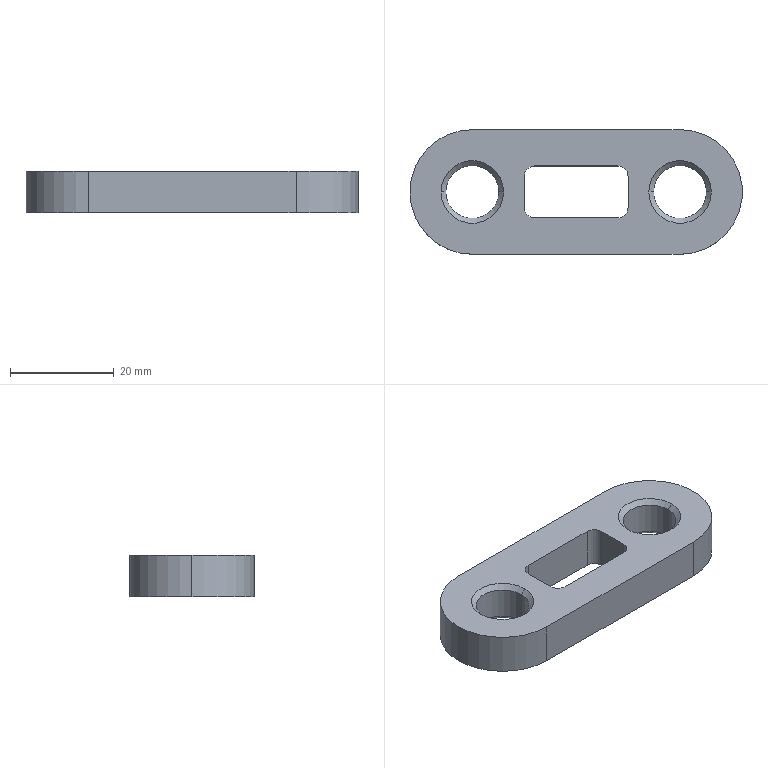Part | SolidWorks | features MirrorPattern 2, 3DProfileFeature 1, Extrusion 1, HoleWzd 1 | 1 solid | 27 faces | box 64 x 24 x 8 mm | volume 8361 mm3 | cylinder 11 | cone 8 | plane 8 | commonest cylinder face diameters 4 x4 10.2 x4 24 x3
STEP:
#1=CARTESIAN_POINT('',(45.1,0.,-3.075));
#2=VERTEX_POINT('',#1);
#3=CARTESIAN_POINT('',(34.9,0.,-3.075));
#4=VERTEX_POINT('',#3);
#5=CARTESIAN_POINT('',(40.,0.,-3.075));
#6=DIRECTION('',(0.,0.,-1.));
#7=DIRECTION('',(-1.,0.,0.));
#8=AXIS2_PLACEMENT_3D('',#5,#6,#7);
#9=CIRCLE('',#8,5.1);
#10=EDGE_CURVE('',#2,#4,#9,.T.);
#11=ORIENTED_EDGE('',*,*,#10,.F.);
#12=CARTESIAN_POINT('',(46.025,0.,-4.));
#13=VERTEX_POINT('',#12);
#14=CARTESIAN_POINT('',(46.025,0.,-4.));
#15=DIRECTION('',(0.7071,0.,-0.7071));
#16=VECTOR('',#15,1000.);
#17=LINE('',#14,#16);
#18=EDGE_CURVE('',#2,#13,#17,.T.);
#19=ORIENTED_EDGE('',*,*,#18,.T.);
#20=CARTESIAN_POINT('',(33.975,0.,-4.));
#21=VERTEX_POINT('',#20);
#22=CARTESIAN_POINT('',(40.,0.,-4.));
#23=DIRECTION('',(0.,0.,-1.));
#24=DIRECTION('',(-1.,0.,0.));
#25=AXIS2_PLACEMENT_3D('',#22,#23,#24);
#26=CIRCLE('',#25,6.025);
#27=EDGE_CURVE('',#13,#21,#26,.T.);
#28=ORIENTED_EDGE('',*,*,#27,.T.);
#29=CARTESIAN_POINT('',(33.975,0.,-4.));
#30=DIRECTION('',(-0.7071,0.,-0.7071));
#31=VECTOR('',#30,1000.);
#32=LINE('',#29,#31);
#33=EDGE_CURVE('',#4,#21,#32,.T.);
#34=ORIENTED_EDGE('',*,*,#33,.F.);
#35=EDGE_LOOP('',(#11,#19,#28,#34));
#36=FACE_OUTER_BOUND('',#35,.T.);
#37=CARTESIAN_POINT('',(40.,0.,-4.));
#38=DIRECTION('',(0.,0.,-1.));
#39=DIRECTION('',(-1.,0.,0.));
#40=AXIS2_PLACEMENT_3D('',#37,#38,#39);
#41=CONICAL_SURFACE('',#40,6.025,0.7854);
#42=ADVANCED_FACE('',(#36),#41,.F.);
#43=CARTESIAN_POINT('',(34.9,0.,3.075));
#44=VERTEX_POINT('',#43);
#45=CARTESIAN_POINT('',(45.1,0.,3.075));
#46=VERTEX_POINT('',#45);
#47=CARTESIAN_POINT('',(40.,0.,3.075));
#48=DIRECTION('',(0.,0.,1.));
#49=DIRECTION('',(1.,0.,0.));
#50=AXIS2_PLACEMENT_3D('',#47,#48,#49);
#51=CIRCLE('',#50,5.1);
#52=EDGE_CURVE('',#44,#46,#51,.T.);
#53=ORIENTED_EDGE('',*,*,#52,.F.);
#54=CARTESIAN_POINT('',(33.975,0.,4.));
#55=VERTEX_POINT('',#54);
#56=CARTESIAN_POINT('',(33.975,0.,4.));
#57=DIRECTION('',(-0.7071,0.,0.7071));
#58=VECTOR('',#57,1000.);
#59=LINE('',#56,#58);
#60=EDGE_CURVE('',#44,#55,#59,.T.);
#61=ORIENTED_EDGE('',*,*,#60,.T.);
#62=CARTESIAN_POINT('',(46.025,0.,4.));
#63=VERTEX_POINT('',#62);
#64=CARTESIAN_POINT('',(40.,0.,4.));
#65=DIRECTION('',(0.,0.,1.));
#66=DIRECTION('',(1.,0.,0.));
#67=AXIS2_PLACEMENT_3D('',#64,#65,#66);
#68=CIRCLE('',#67,6.025);
#69=EDGE_CURVE('',#55,#63,#68,.T.);
#70=ORIENTED_EDGE('',*,*,#69,.T.);
#71=CARTESIAN_POINT('',(46.025,0.,4.));
#72=DIRECTION('',(0.7071,0.,0.7071));
#73=VECTOR('',#72,1000.);
#74=LINE('',#71,#73);
#75=EDGE_CURVE('',#46,#63,#74,.T.);
#76=ORIENTED_EDGE('',*,*,#75,.F.);
#77=EDGE_LOOP('',(#53,#61,#70,#76));
#78=FACE_OUTER_BOUND('',#77,.T.);
#79=CARTESIAN_POINT('',(40.,0.,4.));
#80=DIRECTION('',(0.,0.,1.));
#81=DIRECTION('',(1.,0.,0.));
#82=AXIS2_PLACEMENT_3D('',#79,#80,#81);
#83=CONICAL_SURFACE('',#82,6.025,0.7854);
#84=ADVANCED_FACE('',(#78),#83,.F.);
#85=ORIENTED_EDGE('',*,*,#10,.T.);
#86=CARTESIAN_POINT('',(34.9,0.,4.));
#87=DIRECTION('',(0.,0.,1.));
#88=VECTOR('',#87,1000.);
#89=LINE('',#86,#88);
#90=EDGE_CURVE('',#4,#44,#89,.T.);
#91=ORIENTED_EDGE('',*,*,#90,.T.);
#92=ORIENTED_EDGE('',*,*,#52,.T.);
#93=CARTESIAN_POINT('',(45.1,0.,4.));
#94=DIRECTION('',(0.,0.,1.));
#95=VECTOR('',#94,1000.);
#96=LINE('',#93,#95);
#97=EDGE_CURVE('',#2,#46,#96,.T.);
#98=ORIENTED_EDGE('',*,*,#97,.F.);
#99=EDGE_LOOP('',(#85,#91,#92,#98));
#100=FACE_OUTER_BOUND('',#99,.T.);
#101=CARTESIAN_POINT('',(40.,0.,4.));
#102=DIRECTION('',(0.,0.,1.));
#103=DIRECTION('',(1.,0.,0.));
#104=AXIS2_PLACEMENT_3D('',#101,#102,#103);
#105=CYLINDRICAL_SURFACE('',#104,5.1);
#106=ADVANCED_FACE('',(#100),#105,.F.);
#107=CARTESIAN_POINT('',(5.1,0.,-3.075));
#108=VERTEX_POINT('',#107);
#109=CARTESIAN_POINT('',(-5.1,0.,-3.075));
#110=VERTEX_POINT('',#109);
#111=CARTESIAN_POINT('',(0.,0.,-3.075));
#112=DIRECTION('',(0.,0.,-1.));
#113=DIRECTION('',(-1.,0.,0.));
#114=AXIS2_PLACEMENT_3D('',#111,#112,#113);
#115=CIRCLE('',#114,5.1);
#116=EDGE_CURVE('',#108,#110,#115,.T.);
#117=ORIENTED_EDGE('',*,*,#116,.F.);
#118=CARTESIAN_POINT('',(6.025,0.,-4.));
#119=VERTEX_POINT('',#118);
#120=CARTESIAN_POINT('',(6.025,0.,-4.));
#121=DIRECTION('',(0.7071,0.,-0.7071));
#122=VECTOR('',#121,1000.);
#123=LINE('',#120,#122);
#124=EDGE_CURVE('',#108,#119,#123,.T.);
#125=ORIENTED_EDGE('',*,*,#124,.T.);
#126=CARTESIAN_POINT('',(-6.025,0.,-4.));
#127=VERTEX_POINT('',#126);
#128=CARTESIAN_POINT('',(0.,0.,-4.));
#129=DIRECTION('',(0.,0.,-1.));
#130=DIRECTION('',(-1.,0.,0.));
#131=AXIS2_PLACEMENT_3D('',#128,#129,#130);
#132=CIRCLE('',#131,6.025);
#133=EDGE_CURVE('',#119,#127,#132,.T.);
#134=ORIENTED_EDGE('',*,*,#133,.T.);
#135=CARTESIAN_POINT('',(-6.025,0.,-4.));
#136=DIRECTION('',(-0.7071,0.,-0.7071));
#137=VECTOR('',#136,1000.);
#138=LINE('',#135,#137);
#139=EDGE_CURVE('',#110,#127,#138,.T.);
#140=ORIENTED_EDGE('',*,*,#139,.F.);
#141=EDGE_LOOP('',(#117,#125,#134,#140));
#142=FACE_OUTER_BOUND('',#141,.T.);
#143=CARTESIAN_POINT('',(0.,0.,-4.));
#144=DIRECTION('',(0.,0.,-1.));
#145=DIRECTION('',(-1.,0.,0.));
#146=AXIS2_PLACEMENT_3D('',#143,#144,#145);
#147=CONICAL_SURFACE('',#146,6.025,0.7854);
#148=ADVANCED_FACE('',(#142),#147,.F.);
#149=CARTESIAN_POINT('',(-5.1,0.,3.075));
#150=VERTEX_POINT('',#149);
#151=CARTESIAN_POINT('',(5.1,0.,3.075));
#152=VERTEX_POINT('',#151);
#153=CARTESIAN_POINT('',(0.,0.,3.075));
#154=DIRECTION('',(0.,0.,1.));
#155=DIRECTION('',(1.,0.,0.));
#156=AXIS2_PLACEMENT_3D('',#153,#154,#155);
#157=CIRCLE('',#156,5.1);
#158=EDGE_CURVE('',#150,#152,#157,.T.);
#159=ORIENTED_EDGE('',*,*,#158,.F.);
#160=CARTESIAN_POINT('',(-6.025,0.,4.));
#161=VERTEX_POINT('',#160);
#162=CARTESIAN_POINT('',(-6.025,0.,4.));
#163=DIRECTION('',(-0.7071,0.,0.7071));
#164=VECTOR('',#163,1000.);
#165=LINE('',#162,#164);
#166=EDGE_CURVE('',#150,#161,#165,.T.);
#167=ORIENTED_EDGE('',*,*,#166,.T.);
#168=CARTESIAN_POINT('',(6.025,0.,4.));
#169=VERTEX_POINT('',#168);
#170=CARTESIAN_POINT('',(0.,0.,4.));
#171=DIRECTION('',(0.,0.,1.));
#172=DIRECTION('',(1.,0.,0.));
#173=AXIS2_PLACEMENT_3D('',#170,#171,#172);
#174=CIRCLE('',#173,6.025);
#175=EDGE_CURVE('',#161,#169,#174,.T.);
#176=ORIENTED_EDGE('',*,*,#175,.T.);
#177=CARTESIAN_POINT('',(6.025,0.,4.));
#178=DIRECTION('',(0.7071,0.,0.7071));
#179=VECTOR('',#178,1000.);
#180=LINE('',#177,#179);
#181=EDGE_CURVE('',#152,#169,#180,.T.);
#182=ORIENTED_EDGE('',*,*,#181,.F.);
#183=EDGE_LOOP('',(#159,#167,#176,#182));
#184=FACE_OUTER_BOUND('',#183,.T.);
#185=CARTESIAN_POINT('',(0.,0.,4.));
#186=DIRECTION('',(0.,0.,1.));
#187=DIRECTION('',(1.,0.,0.));
#188=AXIS2_PLACEMENT_3D('',#185,#186,#187);
#189=CONICAL_SURFACE('',#188,6.025,0.7854);
#190=ADVANCED_FACE('',(#184),#189,.F.);
#191=ORIENTED_EDGE('',*,*,#116,.T.);
#192=CARTESIAN_POINT('',(-5.1,0.,4.));
#193=DIRECTION('',(0.,0.,1.));
#194=VECTOR('',#193,1000.);
#195=LINE('',#192,#194);
#196=EDGE_CURVE('',#110,#150,#195,.T.);
#197=ORIENTED_EDGE('',*,*,#196,.T.);
#198=ORIENTED_EDGE('',*,*,#158,.T.);
#199=CARTESIAN_POINT('',(5.1,0.,4.));
#200=DIRECTION('',(0.,0.,1.));
#201=VECTOR('',#200,1000.);
#202=LINE('',#199,#201);
#203=EDGE_CURVE('',#108,#152,#202,.T.);
#204=ORIENTED_EDGE('',*,*,#203,.F.);
#205=EDGE_LOOP('',(#191,#197,#198,#204));
#206=FACE_OUTER_BOUND('',#205,.T.);
#207=CARTESIAN_POINT('',(0.,0.,4.));
#208=DIRECTION('',(0.,0.,1.));
#209=DIRECTION('',(1.,0.,0.));
#210=AXIS2_PLACEMENT_3D('',#207,#208,#209);
#211=CYLINDRICAL_SURFACE('',#210,5.1);
#212=ADVANCED_FACE('',(#206),#211,.F.);
#213=CARTESIAN_POINT('',(-12.,0.,4.));
#214=VERTEX_POINT('',#213);
#215=CARTESIAN_POINT('',(0.,-12.,4.));
#216=VERTEX_POINT('',#215);
#217=CARTESIAN_POINT('',(0.,0.,4.));
#218=DIRECTION('',(0.,0.,1.));
#219=DIRECTION('',(1.,0.,0.));
#220=AXIS2_PLACEMENT_3D('',#217,#218,#219);
#221=CIRCLE('',#220,12.);
#222=EDGE_CURVE('',#214,#216,#221,.T.);
#223=ORIENTED_EDGE('',*,*,#222,.F.);
#224=CARTESIAN_POINT('',(-12.,0.,-4.));
#225=VERTEX_POINT('',#224);
#226=CARTESIAN_POINT('',(-12.,0.,4.));
#227=DIRECTION('',(0.,0.,-1.));
#228=VECTOR('',#227,1000.);
#229=LINE('',#226,#228);
#230=EDGE_CURVE('',#214,#225,#229,.T.);
#231=ORIENTED_EDGE('',*,*,#230,.T.);
#232=CARTESIAN_POINT('',(0.,-12.,-4.));
#233=VERTEX_POINT('',#232);
#234=CARTESIAN_POINT('',(0.,0.,-4.));
#235=DIRECTION('',(0.,0.,1.));
#236=DIRECTION('',(1.,0.,0.));
#237=AXIS2_PLACEMENT_3D('',#234,#235,#236);
#238=CIRCLE('',#237,12.);
#239=EDGE_CURVE('',#225,#233,#238,.T.);
#240=ORIENTED_EDGE('',*,*,#239,.T.);
#241=CARTESIAN_POINT('',(0.,-12.,4.));
#242=DIRECTION('',(0.,0.,-1.));
#243=VECTOR('',#242,1000.);
#244=LINE('',#241,#243);
#245=EDGE_CURVE('',#216,#233,#244,.T.);
#246=ORIENTED_EDGE('',*,*,#245,.F.);
#247=EDGE_LOOP('',(#223,#231,#240,#246));
#248=FACE_OUTER_BOUND('',#247,.T.);
#249=CARTESIAN_POINT('',(0.,0.,4.));
#250=DIRECTION('',(0.,0.,-1.));
#251=DIRECTION('',(-1.,0.,0.));
#252=AXIS2_PLACEMENT_3D('',#249,#250,#251);
#253=CYLINDRICAL_SURFACE('',#252,12.);
#254=ADVANCED_FACE('',(#248),#253,.T.);
#255=CARTESIAN_POINT('',(0.,0.,-4.));
#256=DIRECTION('',(0.,0.,-1.));
#257=DIRECTION('',(-1.,0.,0.));
#258=AXIS2_PLACEMENT_3D('',#255,#256,#257);
#259=CIRCLE('',#258,6.025);
#260=EDGE_CURVE('',#127,#119,#259,.T.);
#261=ORIENTED_EDGE('',*,*,#260,.F.);
#262=ORIENTED_EDGE('',*,*,#133,.F.);
#263=EDGE_LOOP('',(#261,#262));
#264=FACE_BOUND('',#263,.T.);
#265=CARTESIAN_POINT('',(0.,12.,-4.));
#266=VERTEX_POINT('',#265);
#267=CARTESIAN_POINT('',(0.,0.,-4.));
#268=DIRECTION('',(0.,0.,1.));
#269=DIRECTION('',(1.,0.,0.));
#270=AXIS2_PLACEMENT_3D('',#267,#268,#269);
#271=CIRCLE('',#270,12.);
#272=EDGE_CURVE('',#266,#225,#271,.T.);
#273=ORIENTED_EDGE('',*,*,#272,.F.);
#274=CARTESIAN_POINT('',(40.,12.,-4.));
#275=VERTEX_POINT('',#274);
#276=CARTESIAN_POINT('',(0.,12.,-4.));
#277=DIRECTION('',(-1.,0.,0.));
#278=VECTOR('',#277,1000.);
#279=LINE('',#276,#278);
#280=EDGE_CURVE('',#275,#266,#279,.T.);
#281=ORIENTED_EDGE('',*,*,#280,.F.);
#282=CARTESIAN_POINT('',(40.,-12.,-4.));
#283=VERTEX_POINT('',#282);
#284=CARTESIAN_POINT('',(40.,0.,-4.));
#285=DIRECTION('',(0.,0.,1.));
#286=DIRECTION('',(1.,0.,0.));
#287=AXIS2_PLACEMENT_3D('',#284,#285,#286);
#288=CIRCLE('',#287,12.);
#289=EDGE_CURVE('',#283,#275,#288,.T.);
#290=ORIENTED_EDGE('',*,*,#289,.F.);
#291=CARTESIAN_POINT('',(0.,-12.,-4.));
#292=DIRECTION('',(1.,0.,0.));
#293=VECTOR('',#292,1000.);
#294=LINE('',#291,#293);
#295=EDGE_CURVE('',#233,#283,#294,.T.);
#296=ORIENTED_EDGE('',*,*,#295,.F.);
#297=ORIENTED_EDGE('',*,*,#239,.F.);
#298=EDGE_LOOP('',(#273,#281,#290,#296,#297));
#299=FACE_OUTER_BOUND('',#298,.T.);
#300=CARTESIAN_POINT('',(30.,3.,-4.));
#301=VERTEX_POINT('',#300);
#302=CARTESIAN_POINT('',(28.,5.,-4.));
#303=VERTEX_POINT('',#302);
#304=CARTESIAN_POINT('',(28.,3.,-4.));
#305=DIRECTION('',(0.,0.,1.));
#306=DIRECTION('',(-1.,0.,0.));
#307=AXIS2_PLACEMENT_3D('',#304,#305,#306);
#308=CIRCLE('',#307,2.);
#309=EDGE_CURVE('',#301,#303,#308,.T.);
#310=ORIENTED_EDGE('',*,*,#309,.T.);
#311=CARTESIAN_POINT('',(12.,5.,-4.));
#312=VERTEX_POINT('',#311);
#313=CARTESIAN_POINT('',(12.,5.,-4.));
#314=DIRECTION('',(-1.,0.,0.));
#315=VECTOR('',#314,1000.);
#316=LINE('',#313,#315);
#317=EDGE_CURVE('',#303,#312,#316,.T.);
#318=ORIENTED_EDGE('',*,*,#317,.T.);
#319=CARTESIAN_POINT('',(10.,3.,-4.));
#320=VERTEX_POINT('',#319);
#321=CARTESIAN_POINT('',(12.,3.,-4.));
#322=DIRECTION('',(0.,0.,1.));
#323=DIRECTION('',(-1.,0.,0.));
#324=AXIS2_PLACEMENT_3D('',#321,#322,#323);
#325=CIRCLE('',#324,2.);
#326=EDGE_CURVE('',#312,#320,#325,.T.);
#327=ORIENTED_EDGE('',*,*,#326,.T.);
#328=CARTESIAN_POINT('',(10.,-3.,-4.));
#329=VERTEX_POINT('',#328);
#330=CARTESIAN_POINT('',(10.,-3.,-4.));
#331=DIRECTION('',(0.,-1.,0.));
#332=VECTOR('',#331,1000.);
#333=LINE('',#330,#332);
#334=EDGE_CURVE('',#320,#329,#333,.T.);
#335=ORIENTED_EDGE('',*,*,#334,.T.);
#336=CARTESIAN_POINT('',(12.,-5.,-4.));
#337=VERTEX_POINT('',#336);
#338=CARTESIAN_POINT('',(12.,-3.,-4.));
#339=DIRECTION('',(0.,0.,1.));
#340=DIRECTION('',(-1.,0.,0.));
#341=AXIS2_PLACEMENT_3D('',#338,#339,#340);
#342=CIRCLE('',#341,2.);
#343=EDGE_CURVE('',#329,#337,#342,.T.);
#344=ORIENTED_EDGE('',*,*,#343,.T.);
#345=CARTESIAN_POINT('',(28.,-5.,-4.));
#346=VERTEX_POINT('',#345);
#347=CARTESIAN_POINT('',(12.,-5.,-4.));
#348=DIRECTION('',(1.,0.,0.));
#349=VECTOR('',#348,1000.);
#350=LINE('',#347,#349);
#351=EDGE_CURVE('',#337,#346,#350,.T.);
#352=ORIENTED_EDGE('',*,*,#351,.T.);
#353=CARTESIAN_POINT('',(30.,-3.,-4.));
#354=VERTEX_POINT('',#353);
#355=CARTESIAN_POINT('',(28.,-3.,-4.));
#356=DIRECTION('',(0.,0.,1.));
#357=DIRECTION('',(1.,0.,0.));
#358=AXIS2_PLACEMENT_3D('',#355,#356,#357);
#359=CIRCLE('',#358,2.);
#360=EDGE_CURVE('',#346,#354,#359,.T.);
#361=ORIENTED_EDGE('',*,*,#360,.T.);
#362=CARTESIAN_POINT('',(30.,-3.,-4.));
#363=DIRECTION('',(0.,1.,0.));
#364=VECTOR('',#363,1000.);
#365=LINE('',#362,#364);
#366=EDGE_CURVE('',#354,#301,#365,.T.);
#367=ORIENTED_EDGE('',*,*,#366,.T.);
#368=EDGE_LOOP('',(#310,#318,#327,#335,#344,#352,#361,#367));
#369=FACE_BOUND('',#368,.T.);
#370=CARTESIAN_POINT('',(40.,0.,-4.));
#371=DIRECTION('',(0.,0.,-1.));
#372=DIRECTION('',(-1.,0.,0.));
#373=AXIS2_PLACEMENT_3D('',#370,#371,#372);
#374=CIRCLE('',#373,6.025);
#375=EDGE_CURVE('',#21,#13,#374,.T.);
#376=ORIENTED_EDGE('',*,*,#375,.F.);
#377=ORIENTED_EDGE('',*,*,#27,.F.);
#378=EDGE_LOOP('',(#376,#377));
#379=FACE_BOUND('',#378,.T.);
#380=CARTESIAN_POINT('',(0.,0.,-4.));
#381=DIRECTION('',(0.,0.,1.));
#382=DIRECTION('',(1.,0.,0.));
#383=AXIS2_PLACEMENT_3D('',#380,#381,#382);
#384=PLANE('',#383);
#385=ADVANCED_FACE('',(#264,#299,#369,#379),#384,.F.);
#386=CARTESIAN_POINT('',(40.,0.,4.));
#387=DIRECTION('',(0.,0.,1.));
#388=DIRECTION('',(1.,0.,0.));
#389=AXIS2_PLACEMENT_3D('',#386,#387,#388);
#390=CIRCLE('',#389,6.025);
#391=EDGE_CURVE('',#63,#55,#390,.T.);
#392=ORIENTED_EDGE('',*,*,#391,.F.);
#393=ORIENTED_EDGE('',*,*,#69,.F.);
#394=EDGE_LOOP('',(#392,#393));
#395=FACE_BOUND('',#394,.T.);
#396=CARTESIAN_POINT('',(0.,0.,4.));
#397=DIRECTION('',(0.,0.,1.));
#398=DIRECTION('',(1.,0.,0.));
#399=AXIS2_PLACEMENT_3D('',#396,#397,#398);
#400=CIRCLE('',#399,6.025);
#401=EDGE_CURVE('',#169,#161,#400,.T.);
#402=ORIENTED_EDGE('',*,*,#401,.F.);
#403=ORIENTED_EDGE('',*,*,#175,.F.);
#404=EDGE_LOOP('',(#402,#403));
#405=FACE_BOUND('',#404,.T.);
#406=CARTESIAN_POINT('',(0.,12.,4.));
#407=VERTEX_POINT('',#406);
#408=CARTESIAN_POINT('',(0.,0.,4.));
#409=DIRECTION('',(0.,0.,1.));
#410=DIRECTION('',(1.,0.,0.));
#411=AXIS2_PLACEMENT_3D('',#408,#409,#410);
#412=CIRCLE('',#411,12.);
#413=EDGE_CURVE('',#407,#214,#412,.T.);
#414=ORIENTED_EDGE('',*,*,#413,.T.);
#415=ORIENTED_EDGE('',*,*,#222,.T.);
#416=CARTESIAN_POINT('',(40.,-12.,4.));
#417=VERTEX_POINT('',#416);
#418=CARTESIAN_POINT('',(0.,-12.,4.));
#419=DIRECTION('',(1.,0.,0.));
#420=VECTOR('',#419,1000.);
#421=LINE('',#418,#420);
#422=EDGE_CURVE('',#216,#417,#421,.T.);
#423=ORIENTED_EDGE('',*,*,#422,.T.);
#424=CARTESIAN_POINT('',(40.,12.,4.));
#425=VERTEX_POINT('',#424);
#426=CARTESIAN_POINT('',(40.,0.,4.));
#427=DIRECTION('',(0.,0.,1.));
#428=DIRECTION('',(1.,0.,0.));
#429=AXIS2_PLACEMENT_3D('',#426,#427,#428);
#430=CIRCLE('',#429,12.);
#431=EDGE_CURVE('',#417,#425,#430,.T.);
#432=ORIENTED_EDGE('',*,*,#431,.T.);
#433=CARTESIAN_POINT('',(0.,12.,4.));
#434=DIRECTION('',(-1.,0.,0.));
#435=VECTOR('',#434,1000.);
#436=LINE('',#433,#435);
#437=EDGE_CURVE('',#425,#407,#436,.T.);
#438=ORIENTED_EDGE('',*,*,#437,.T.);
#439=EDGE_LOOP('',(#414,#415,#423,#432,#438));
#440=FACE_OUTER_BOUND('',#439,.T.);
#441=CARTESIAN_POINT('',(28.,5.,4.));
#442=VERTEX_POINT('',#441);
#443=CARTESIAN_POINT('',(12.,5.,4.));
#444=VERTEX_POINT('',#443);
#445=CARTESIAN_POINT('',(12.,5.,4.));
#446=DIRECTION('',(-1.,0.,0.));
#447=VECTOR('',#446,1000.);
#448=LINE('',#445,#447);
#449=EDGE_CURVE('',#442,#444,#448,.T.);
#450=ORIENTED_EDGE('',*,*,#449,.F.);
#451=CARTESIAN_POINT('',(30.,3.,4.));
#452=VERTEX_POINT('',#451);
#453=CARTESIAN_POINT('',(28.,3.,4.));
#454=DIRECTION('',(0.,0.,1.));
#455=DIRECTION('',(-1.,0.,0.));
#456=AXIS2_PLACEMENT_3D('',#453,#454,#455);
#457=CIRCLE('',#456,2.);
#458=EDGE_CURVE('',#452,#442,#457,.T.);
#459=ORIENTED_EDGE('',*,*,#458,.F.);
#460=CARTESIAN_POINT('',(30.,-3.,4.));
#461=VERTEX_POINT('',#460);
#462=CARTESIAN_POINT('',(30.,-3.,4.));
#463=DIRECTION('',(0.,1.,0.));
#464=VECTOR('',#463,1000.);
#465=LINE('',#462,#464);
#466=EDGE_CURVE('',#461,#452,#465,.T.);
#467=ORIENTED_EDGE('',*,*,#466,.F.);
#468=CARTESIAN_POINT('',(28.,-5.,4.));
#469=VERTEX_POINT('',#468);
#470=CARTESIAN_POINT('',(28.,-3.,4.));
#471=DIRECTION('',(0.,0.,1.));
#472=DIRECTION('',(1.,0.,0.));
#473=AXIS2_PLACEMENT_3D('',#470,#471,#472);
#474=CIRCLE('',#473,2.);
#475=EDGE_CURVE('',#469,#461,#474,.T.);
#476=ORIENTED_EDGE('',*,*,#475,.F.);
#477=CARTESIAN_POINT('',(12.,-5.,4.));
#478=VERTEX_POINT('',#477);
#479=CARTESIAN_POINT('',(12.,-5.,4.));
#480=DIRECTION('',(1.,0.,0.));
#481=VECTOR('',#480,1000.);
#482=LINE('',#479,#481);
#483=EDGE_CURVE('',#478,#469,#482,.T.);
#484=ORIENTED_EDGE('',*,*,#483,.F.);
#485=CARTESIAN_POINT('',(10.,-3.,4.));
#486=VERTEX_POINT('',#485);
#487=CARTESIAN_POINT('',(12.,-3.,4.));
#488=DIRECTION('',(0.,0.,1.));
#489=DIRECTION('',(-1.,0.,0.));
#490=AXIS2_PLACEMENT_3D('',#487,#488,#489);
#491=CIRCLE('',#490,2.);
#492=EDGE_CURVE('',#486,#478,#491,.T.);
#493=ORIENTED_EDGE('',*,*,#492,.F.);
#494=CARTESIAN_POINT('',(10.,3.,4.));
#495=VERTEX_POINT('',#494);
#496=CARTESIAN_POINT('',(10.,-3.,4.));
#497=DIRECTION('',(0.,-1.,0.));
#498=VECTOR('',#497,1000.);
#499=LINE('',#496,#498);
#500=EDGE_CURVE('',#495,#486,#499,.T.);
#501=ORIENTED_EDGE('',*,*,#500,.F.);
#502=CARTESIAN_POINT('',(12.,3.,4.));
#503=DIRECTION('',(0.,0.,1.));
#504=DIRECTION('',(-1.,0.,0.));
#505=AXIS2_PLACEMENT_3D('',#502,#503,#504);
#506=CIRCLE('',#505,2.);
#507=EDGE_CURVE('',#444,#495,#506,.T.);
#508=ORIENTED_EDGE('',*,*,#507,.F.);
#509=EDGE_LOOP('',(#450,#459,#467,#476,#484,#493,#501,#508));
#510=FACE_BOUND('',#509,.T.);
#511=CARTESIAN_POINT('',(0.,0.,4.));
#512=DIRECTION('',(0.,0.,1.));
#513=DIRECTION('',(1.,0.,0.));
#514=AXIS2_PLACEMENT_3D('',#511,#512,#513);
#515=PLANE('',#514);
#516=ADVANCED_FACE('',(#395,#405,#440,#510),#515,.T.);
#517=ORIENTED_EDGE('',*,*,#230,.F.);
#518=ORIENTED_EDGE('',*,*,#413,.F.);
#519=CARTESIAN_POINT('',(0.,12.,4.));
#520=DIRECTION('',(0.,0.,-1.));
#521=VECTOR('',#520,1000.);
#522=LINE('',#519,#521);
#523=EDGE_CURVE('',#407,#266,#522,.T.);
#524=ORIENTED_EDGE('',*,*,#523,.T.);
#525=ORIENTED_EDGE('',*,*,#272,.T.);
#526=EDGE_LOOP('',(#517,#518,#524,#525));
#527=FACE_OUTER_BOUND('',#526,.T.);
#528=CARTESIAN_POINT('',(0.,0.,4.));
#529=DIRECTION('',(0.,0.,-1.));
#530=DIRECTION('',(-1.,0.,0.));
#531=AXIS2_PLACEMENT_3D('',#528,#529,#530);
#532=CYLINDRICAL_SURFACE('',#531,12.);
#533=ADVANCED_FACE('',(#527),#532,.T.);
#534=ORIENTED_EDGE('',*,*,#295,.T.);
#535=CARTESIAN_POINT('',(40.,-12.,4.));
#536=DIRECTION('',(0.,0.,-1.));
#537=VECTOR('',#536,1000.);
#538=LINE('',#535,#537);
#539=EDGE_CURVE('',#417,#283,#538,.T.);
#540=ORIENTED_EDGE('',*,*,#539,.F.);
#541=ORIENTED_EDGE('',*,*,#422,.F.);
#542=ORIENTED_EDGE('',*,*,#245,.T.);
#543=EDGE_LOOP('',(#534,#540,#541,#542));
#544=FACE_OUTER_BOUND('',#543,.T.);
#545=CARTESIAN_POINT('',(0.,-12.,4.));
#546=DIRECTION('',(0.,1.,0.));
#547=DIRECTION('',(-1.,0.,0.));
#548=AXIS2_PLACEMENT_3D('',#545,#546,#547);
#549=PLANE('',#548);
#550=ADVANCED_FACE('',(#544),#549,.F.);
#551=ORIENTED_EDGE('',*,*,#289,.T.);
#552=CARTESIAN_POINT('',(40.,12.,4.));
#553=DIRECTION('',(0.,0.,-1.));
#554=VECTOR('',#553,1000.);
#555=LINE('',#552,#554);
#556=EDGE_CURVE('',#425,#275,#555,.T.);
#557=ORIENTED_EDGE('',*,*,#556,.F.);
#558=ORIENTED_EDGE('',*,*,#431,.F.);
#559=ORIENTED_EDGE('',*,*,#539,.T.);
#560=EDGE_LOOP('',(#551,#557,#558,#559));
#561=FACE_OUTER_BOUND('',#560,.T.);
#562=CARTESIAN_POINT('',(40.,0.,4.));
#563=DIRECTION('',(0.,0.,-1.));
#564=DIRECTION('',(-1.,0.,0.));
#565=AXIS2_PLACEMENT_3D('',#562,#563,#564);
#566=CYLINDRICAL_SURFACE('',#565,12.);
#567=ADVANCED_FACE('',(#561),#566,.T.);
#568=ORIENTED_EDGE('',*,*,#280,.T.);
#569=ORIENTED_EDGE('',*,*,#523,.F.);
#570=ORIENTED_EDGE('',*,*,#437,.F.);
#571=ORIENTED_EDGE('',*,*,#556,.T.);
#572=EDGE_LOOP('',(#568,#569,#570,#571));
#573=FACE_OUTER_BOUND('',#572,.T.);
#574=CARTESIAN_POINT('',(0.,12.,4.));
#575=DIRECTION('',(0.,-1.,0.));
#576=DIRECTION('',(1.,0.,0.));
#577=AXIS2_PLACEMENT_3D('',#574,#575,#576);
#578=PLANE('',#577);
#579=ADVANCED_FACE('',(#573),#578,.F.);
#580=ORIENTED_EDGE('',*,*,#309,.F.);
#581=CARTESIAN_POINT('',(30.,3.,4.));
#582=DIRECTION('',(0.,0.,-1.));
#583=VECTOR('',#582,1000.);
#584=LINE('',#581,#583);
#585=EDGE_CURVE('',#452,#301,#584,.T.);
#586=ORIENTED_EDGE('',*,*,#585,.F.);
#587=ORIENTED_EDGE('',*,*,#458,.T.);
#588=CARTESIAN_POINT('',(28.,5.,4.));
#589=DIRECTION('',(0.,0.,-1.));
#590=VECTOR('',#589,1000.);
#591=LINE('',#588,#590);
#592=EDGE_CURVE('',#442,#303,#591,.T.);
#593=ORIENTED_EDGE('',*,*,#592,.T.);
#594=EDGE_LOOP('',(#580,#586,#587,#593));
#595=FACE_OUTER_BOUND('',#594,.T.);
#596=CARTESIAN_POINT('',(28.,3.,4.));
#597=DIRECTION('',(0.,0.,-1.));
#598=DIRECTION('',(-1.,0.,0.));
#599=AXIS2_PLACEMENT_3D('',#596,#597,#598);
#600=CYLINDRICAL_SURFACE('',#599,2.);
#601=ADVANCED_FACE('',(#595),#600,.F.);
#602=ORIENTED_EDGE('',*,*,#317,.F.);
#603=ORIENTED_EDGE('',*,*,#592,.F.);
#604=ORIENTED_EDGE('',*,*,#449,.T.);
#605=CARTESIAN_POINT('',(12.,5.,4.));
#606=DIRECTION('',(0.,0.,-1.));
#607=VECTOR('',#606,1000.);
#608=LINE('',#605,#607);
#609=EDGE_CURVE('',#444,#312,#608,.T.);
#610=ORIENTED_EDGE('',*,*,#609,.T.);
#611=EDGE_LOOP('',(#602,#603,#604,#610));
#612=FACE_OUTER_BOUND('',#611,.T.);
#613=CARTESIAN_POINT('',(12.,5.,4.));
#614=DIRECTION('',(0.,-1.,0.));
#615=DIRECTION('',(0.,0.,-1.));
#616=AXIS2_PLACEMENT_3D('',#613,#614,#615);
#617=PLANE('',#616);
#618=ADVANCED_FACE('',(#612),#617,.T.);
#619=ORIENTED_EDGE('',*,*,#326,.F.);
#620=ORIENTED_EDGE('',*,*,#609,.F.);
#621=ORIENTED_EDGE('',*,*,#507,.T.);
#622=CARTESIAN_POINT('',(10.,3.,4.));
#623=DIRECTION('',(0.,0.,-1.));
#624=VECTOR('',#623,1000.);
#625=LINE('',#622,#624);
#626=EDGE_CURVE('',#495,#320,#625,.T.);
#627=ORIENTED_EDGE('',*,*,#626,.T.);
#628=EDGE_LOOP('',(#619,#620,#621,#627));
#629=FACE_OUTER_BOUND('',#628,.T.);
#630=CARTESIAN_POINT('',(12.,3.,4.));
#631=DIRECTION('',(0.,0.,-1.));
#632=DIRECTION('',(-1.,0.,0.));
#633=AXIS2_PLACEMENT_3D('',#630,#631,#632);
#634=CYLINDRICAL_SURFACE('',#633,2.);
#635=ADVANCED_FACE('',(#629),#634,.F.);
#636=ORIENTED_EDGE('',*,*,#334,.F.);
#637=ORIENTED_EDGE('',*,*,#626,.F.);
#638=ORIENTED_EDGE('',*,*,#500,.T.);
#639=CARTESIAN_POINT('',(10.,-3.,4.));
#640=DIRECTION('',(0.,0.,-1.));
#641=VECTOR('',#640,1000.);
#642=LINE('',#639,#641);
#643=EDGE_CURVE('',#486,#329,#642,.T.);
#644=ORIENTED_EDGE('',*,*,#643,.T.);
#645=EDGE_LOOP('',(#636,#637,#638,#644));
#646=FACE_OUTER_BOUND('',#645,.T.);
#647=CARTESIAN_POINT('',(10.,-3.,4.));
#648=DIRECTION('',(1.,0.,0.));
#649=DIRECTION('',(0.,0.,-1.));
#650=AXIS2_PLACEMENT_3D('',#647,#648,#649);
#651=PLANE('',#650);
#652=ADVANCED_FACE('',(#646),#651,.T.);
#653=ORIENTED_EDGE('',*,*,#343,.F.);
#654=ORIENTED_EDGE('',*,*,#643,.F.);
#655=ORIENTED_EDGE('',*,*,#492,.T.);
#656=CARTESIAN_POINT('',(12.,-5.,4.));
#657=DIRECTION('',(0.,0.,-1.));
#658=VECTOR('',#657,1000.);
#659=LINE('',#656,#658);
#660=EDGE_CURVE('',#478,#337,#659,.T.);
#661=ORIENTED_EDGE('',*,*,#660,.T.);
#662=EDGE_LOOP('',(#653,#654,#655,#661));
#663=FACE_OUTER_BOUND('',#662,.T.);
#664=CARTESIAN_POINT('',(12.,-3.,4.));
#665=DIRECTION('',(0.,0.,-1.));
#666=DIRECTION('',(-1.,0.,0.));
#667=AXIS2_PLACEMENT_3D('',#664,#665,#666);
#668=CYLINDRICAL_SURFACE('',#667,2.);
#669=ADVANCED_FACE('',(#663),#668,.F.);
#670=ORIENTED_EDGE('',*,*,#351,.F.);
#671=ORIENTED_EDGE('',*,*,#660,.F.);
#672=ORIENTED_EDGE('',*,*,#483,.T.);
#673=CARTESIAN_POINT('',(28.,-5.,4.));
#674=DIRECTION('',(0.,0.,-1.));
#675=VECTOR('',#674,1000.);
#676=LINE('',#673,#675);
#677=EDGE_CURVE('',#469,#346,#676,.T.);
#678=ORIENTED_EDGE('',*,*,#677,.T.);
#679=EDGE_LOOP('',(#670,#671,#672,#678));
#680=FACE_OUTER_BOUND('',#679,.T.);
#681=CARTESIAN_POINT('',(12.,-5.,4.));
#682=DIRECTION('',(0.,1.,0.));
#683=DIRECTION('',(0.,0.,1.));
#684=AXIS2_PLACEMENT_3D('',#681,#682,#683);
#685=PLANE('',#684);
#686=ADVANCED_FACE('',(#680),#685,.T.);
#687=ORIENTED_EDGE('',*,*,#360,.F.);
#688=ORIENTED_EDGE('',*,*,#677,.F.);
#689=ORIENTED_EDGE('',*,*,#475,.T.);
#690=CARTESIAN_POINT('',(30.,-3.,4.));
#691=DIRECTION('',(0.,0.,-1.));
#692=VECTOR('',#691,1000.);
#693=LINE('',#690,#692);
#694=EDGE_CURVE('',#461,#354,#693,.T.);
#695=ORIENTED_EDGE('',*,*,#694,.T.);
#696=EDGE_LOOP('',(#687,#688,#689,#695));
#697=FACE_OUTER_BOUND('',#696,.T.);
#698=CARTESIAN_POINT('',(28.,-3.,4.));
#699=DIRECTION('',(0.,0.,-1.));
#700=DIRECTION('',(-1.,0.,0.));
#701=AXIS2_PLACEMENT_3D('',#698,#699,#700);
#702=CYLINDRICAL_SURFACE('',#701,2.);
#703=ADVANCED_FACE('',(#697),#702,.F.);
#704=ORIENTED_EDGE('',*,*,#366,.F.);
#705=ORIENTED_EDGE('',*,*,#694,.F.);
#706=ORIENTED_EDGE('',*,*,#466,.T.);
#707=ORIENTED_EDGE('',*,*,#585,.T.);
#708=EDGE_LOOP('',(#704,#705,#706,#707));
#709=FACE_OUTER_BOUND('',#708,.T.);
#710=CARTESIAN_POINT('',(30.,-3.,4.));
#711=DIRECTION('',(-1.,0.,0.));
#712=DIRECTION('',(0.,0.,1.));
#713=AXIS2_PLACEMENT_3D('',#710,#711,#712);
#714=PLANE('',#713);
#715=ADVANCED_FACE('',(#709),#714,.T.);
#716=ORIENTED_EDGE('',*,*,#196,.F.);
#717=CARTESIAN_POINT('',(0.,0.,-3.075));
#718=DIRECTION('',(0.,0.,-1.));
#719=DIRECTION('',(-1.,0.,0.));
#720=AXIS2_PLACEMENT_3D('',#717,#718,#719);
#721=CIRCLE('',#720,5.1);
#722=EDGE_CURVE('',#110,#108,#721,.T.);
#723=ORIENTED_EDGE('',*,*,#722,.T.);
#724=ORIENTED_EDGE('',*,*,#203,.T.);
#725=CARTESIAN_POINT('',(0.,0.,3.075));
#726=DIRECTION('',(0.,0.,1.));
#727=DIRECTION('',(1.,0.,0.));
#728=AXIS2_PLACEMENT_3D('',#725,#726,#727);
#729=CIRCLE('',#728,5.1);
#730=EDGE_CURVE('',#152,#150,#729,.T.);
#731=ORIENTED_EDGE('',*,*,#730,.T.);
#732=EDGE_LOOP('',(#716,#723,#724,#731));
#733=FACE_OUTER_BOUND('',#732,.T.);
#734=CARTESIAN_POINT('',(0.,0.,4.));
#735=DIRECTION('',(0.,0.,1.));
#736=DIRECTION('',(1.,0.,0.));
#737=AXIS2_PLACEMENT_3D('',#734,#735,#736);
#738=CYLINDRICAL_SURFACE('',#737,5.1);
#739=ADVANCED_FACE('',(#733),#738,.F.);
#740=ORIENTED_EDGE('',*,*,#166,.F.);
#741=ORIENTED_EDGE('',*,*,#730,.F.);
#742=ORIENTED_EDGE('',*,*,#181,.T.);
#743=ORIENTED_EDGE('',*,*,#401,.T.);
#744=EDGE_LOOP('',(#740,#741,#742,#743));
#745=FACE_OUTER_BOUND('',#744,.T.);
#746=CARTESIAN_POINT('',(0.,0.,4.));
#747=DIRECTION('',(0.,0.,1.));
#748=DIRECTION('',(1.,0.,0.));
#749=AXIS2_PLACEMENT_3D('',#746,#747,#748);
#750=CONICAL_SURFACE('',#749,6.025,0.7854);
#751=ADVANCED_FACE('',(#745),#750,.F.);
#752=ORIENTED_EDGE('',*,*,#124,.F.);
#753=ORIENTED_EDGE('',*,*,#722,.F.);
#754=ORIENTED_EDGE('',*,*,#139,.T.);
#755=ORIENTED_EDGE('',*,*,#260,.T.);
#756=EDGE_LOOP('',(#752,#753,#754,#755));
#757=FACE_OUTER_BOUND('',#756,.T.);
#758=CARTESIAN_POINT('',(0.,0.,-4.));
#759=DIRECTION('',(0.,0.,-1.));
#760=DIRECTION('',(-1.,0.,0.));
#761=AXIS2_PLACEMENT_3D('',#758,#759,#760);
#762=CONICAL_SURFACE('',#761,6.025,0.7854);
#763=ADVANCED_FACE('',(#757),#762,.F.);
#764=ORIENTED_EDGE('',*,*,#90,.F.);
#765=CARTESIAN_POINT('',(40.,0.,-3.075));
#766=DIRECTION('',(0.,0.,-1.));
#767=DIRECTION('',(-1.,0.,0.));
#768=AXIS2_PLACEMENT_3D('',#765,#766,#767);
#769=CIRCLE('',#768,5.1);
#770=EDGE_CURVE('',#4,#2,#769,.T.);
#771=ORIENTED_EDGE('',*,*,#770,.T.);
#772=ORIENTED_EDGE('',*,*,#97,.T.);
#773=CARTESIAN_POINT('',(40.,0.,3.075));
#774=DIRECTION('',(0.,0.,1.));
#775=DIRECTION('',(1.,0.,0.));
#776=AXIS2_PLACEMENT_3D('',#773,#774,#775);
#777=CIRCLE('',#776,5.1);
#778=EDGE_CURVE('',#46,#44,#777,.T.);
#779=ORIENTED_EDGE('',*,*,#778,.T.);
#780=EDGE_LOOP('',(#764,#771,#772,#779));
#781=FACE_OUTER_BOUND('',#780,.T.);
#782=CARTESIAN_POINT('',(40.,0.,4.));
#783=DIRECTION('',(0.,0.,1.));
#784=DIRECTION('',(1.,0.,0.));
#785=AXIS2_PLACEMENT_3D('',#782,#783,#784);
#786=CYLINDRICAL_SURFACE('',#785,5.1);
#787=ADVANCED_FACE('',(#781),#786,.F.);
#788=ORIENTED_EDGE('',*,*,#60,.F.);
#789=ORIENTED_EDGE('',*,*,#778,.F.);
#790=ORIENTED_EDGE('',*,*,#75,.T.);
#791=ORIENTED_EDGE('',*,*,#391,.T.);
#792=EDGE_LOOP('',(#788,#789,#790,#791));
#793=FACE_OUTER_BOUND('',#792,.T.);
#794=CARTESIAN_POINT('',(40.,0.,4.));
#795=DIRECTION('',(0.,0.,1.));
#796=DIRECTION('',(1.,0.,0.));
#797=AXIS2_PLACEMENT_3D('',#794,#795,#796);
#798=CONICAL_SURFACE('',#797,6.025,0.7854);
#799=ADVANCED_FACE('',(#793),#798,.F.);
#800=ORIENTED_EDGE('',*,*,#18,.F.);
#801=ORIENTED_EDGE('',*,*,#770,.F.);
#802=ORIENTED_EDGE('',*,*,#33,.T.);
#803=ORIENTED_EDGE('',*,*,#375,.T.);
#804=EDGE_LOOP('',(#800,#801,#802,#803));
#805=FACE_OUTER_BOUND('',#804,.T.);
#806=CARTESIAN_POINT('',(40.,0.,-4.));
#807=DIRECTION('',(0.,0.,-1.));
#808=DIRECTION('',(-1.,0.,0.));
#809=AXIS2_PLACEMENT_3D('',#806,#807,#808);
#810=CONICAL_SURFACE('',#809,6.025,0.7854);
#811=ADVANCED_FACE('',(#805),#810,.F.);
#812=CLOSED_SHELL('',(#42,#84,#106,#148,#190,#212,#254,#385,#516,#533,#550,#567,#579,#601,#618,#635,#652,#669,#686,#703,#715,#739,#751,#763,#787,#799,#811));
#813=MANIFOLD_SOLID_BREP('',#812);
#814=CARTESIAN_POINT('',(0.,0.,0.));
#815=DIRECTION('',(0.,0.,1.));
#816=DIRECTION('',(1.,0.,0.));
#817=AXIS2_PLACEMENT_3D('',#814,#815,#816);
#818=(LENGTH_UNIT()NAMED_UNIT(*)SI_UNIT(.MILLI.,.METRE.));
#819=UNCERTAINTY_MEASURE_WITH_UNIT(LENGTH_MEASURE(0.00001),#818,'','');
#820=(NAMED_UNIT(*)PLANE_ANGLE_UNIT()SI_UNIT($,.RADIAN.));
#821=(NAMED_UNIT(*)SI_UNIT($,.STERADIAN.)SOLID_ANGLE_UNIT());
#822=(GEOMETRIC_REPRESENTATION_CONTEXT(3)GLOBAL_UNCERTAINTY_ASSIGNED_CONTEXT((#819))GLOBAL_UNIT_ASSIGNED_CONTEXT((#818,#820,#821))REPRESENTATION_CONTEXT('',''));
#823=ADVANCED_BREP_SHAPE_REPRESENTATION('',(#813,#817),#822);